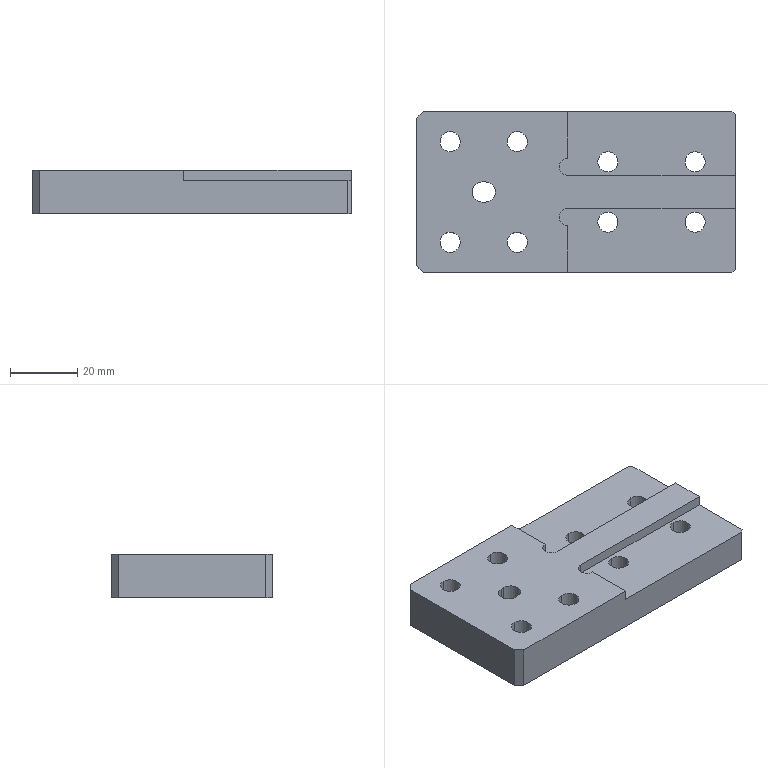Part | STEP file | J454-EBZ05-19-00-Part-1-4 | 1 solid | 38 faces | box 95 x 48 x 13 mm | volume 50412 mm3 | cylinder 20 | plane 18 | commonest cylinder face diameters 6 x18 5 x2